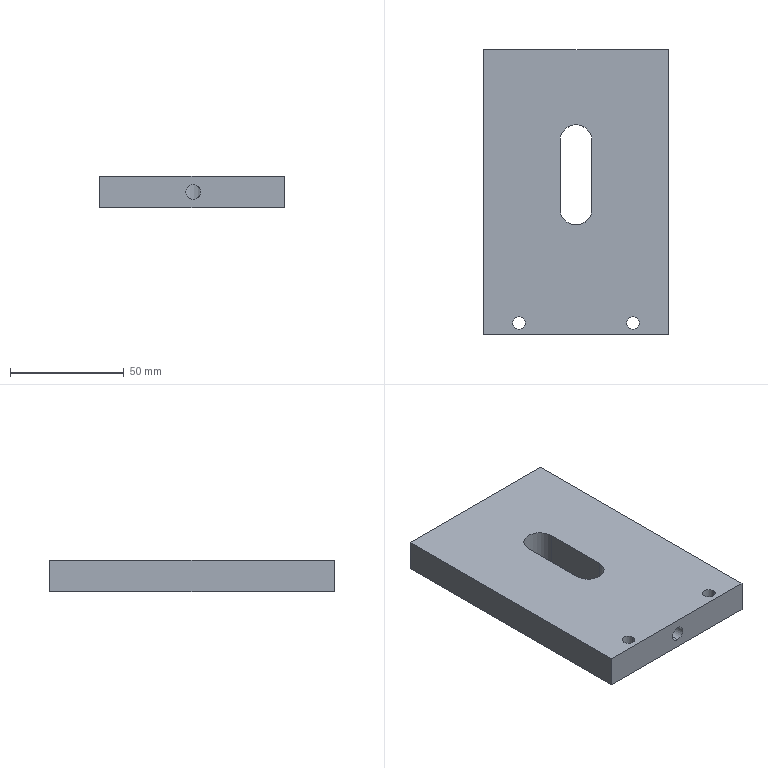Part | SolidWorks | features ICE 2, Cut 1, Extrusion 1, HoleWzd 1 | 1 solid | 24 faces | box 81 x 125 x 14 mm | volume 129784 mm3 | cylinder 12 | plane 8 | cone 4 | commonest cylinder face diameters 5.5 x4 6.8 x4 6.5 x2 14 x2
STEP:
#1=CARTESIAN_POINT('',(62.75,-120.,0.));
#2=VERTEX_POINT('',#1);
#3=CARTESIAN_POINT('',(68.25,-120.,0.));
#4=VERTEX_POINT('',#3);
#5=CARTESIAN_POINT('',(65.5,-120.,0.));
#6=DIRECTION('',(0.,0.,1.));
#7=DIRECTION('',(1.,0.,0.));
#8=AXIS2_PLACEMENT_3D('',#5,#6,#7);
#9=CIRCLE('',#8,2.75);
#10=EDGE_CURVE('',#2,#4,#9,.T.);
#11=ORIENTED_EDGE('',*,*,#10,.F.);
#12=CARTESIAN_POINT('',(62.75,-120.,14.));
#13=VERTEX_POINT('',#12);
#14=CARTESIAN_POINT('',(62.75,-120.,0.));
#15=DIRECTION('',(0.,0.,1.));
#16=VECTOR('',#15,1000.);
#17=LINE('',#14,#16);
#18=EDGE_CURVE('',#2,#13,#17,.T.);
#19=ORIENTED_EDGE('',*,*,#18,.T.);
#20=CARTESIAN_POINT('',(68.25,-120.,14.));
#21=VERTEX_POINT('',#20);
#22=CARTESIAN_POINT('',(65.5,-120.,14.));
#23=DIRECTION('',(0.,0.,1.));
#24=DIRECTION('',(1.,0.,0.));
#25=AXIS2_PLACEMENT_3D('',#22,#23,#24);
#26=CIRCLE('',#25,2.75);
#27=EDGE_CURVE('',#13,#21,#26,.T.);
#28=ORIENTED_EDGE('',*,*,#27,.T.);
#29=CARTESIAN_POINT('',(68.25,-120.,0.));
#30=DIRECTION('',(0.,0.,1.));
#31=VECTOR('',#30,1000.);
#32=LINE('',#29,#31);
#33=EDGE_CURVE('',#4,#21,#32,.T.);
#34=ORIENTED_EDGE('',*,*,#33,.F.);
#35=EDGE_LOOP('',(#11,#19,#28,#34));
#36=FACE_OUTER_BOUND('',#35,.T.);
#37=CARTESIAN_POINT('',(65.5,-120.,0.));
#38=DIRECTION('',(0.,0.,1.));
#39=DIRECTION('',(1.,0.,0.));
#40=AXIS2_PLACEMENT_3D('',#37,#38,#39);
#41=CYLINDRICAL_SURFACE('',#40,2.75);
#42=ADVANCED_FACE('',(#36),#41,.F.);
#43=CARTESIAN_POINT('',(12.75,-120.,0.));
#44=VERTEX_POINT('',#43);
#45=CARTESIAN_POINT('',(18.25,-120.,0.));
#46=VERTEX_POINT('',#45);
#47=CARTESIAN_POINT('',(15.5,-120.,0.));
#48=DIRECTION('',(0.,0.,1.));
#49=DIRECTION('',(1.,0.,0.));
#50=AXIS2_PLACEMENT_3D('',#47,#48,#49);
#51=CIRCLE('',#50,2.75);
#52=EDGE_CURVE('',#44,#46,#51,.T.);
#53=ORIENTED_EDGE('',*,*,#52,.F.);
#54=CARTESIAN_POINT('',(12.75,-120.,14.));
#55=VERTEX_POINT('',#54);
#56=CARTESIAN_POINT('',(12.75,-120.,0.));
#57=DIRECTION('',(0.,0.,1.));
#58=VECTOR('',#57,1000.);
#59=LINE('',#56,#58);
#60=EDGE_CURVE('',#44,#55,#59,.T.);
#61=ORIENTED_EDGE('',*,*,#60,.T.);
#62=CARTESIAN_POINT('',(18.25,-120.,14.));
#63=VERTEX_POINT('',#62);
#64=CARTESIAN_POINT('',(15.5,-120.,14.));
#65=DIRECTION('',(0.,0.,1.));
#66=DIRECTION('',(1.,0.,0.));
#67=AXIS2_PLACEMENT_3D('',#64,#65,#66);
#68=CIRCLE('',#67,2.75);
#69=EDGE_CURVE('',#55,#63,#68,.T.);
#70=ORIENTED_EDGE('',*,*,#69,.T.);
#71=CARTESIAN_POINT('',(18.25,-120.,0.));
#72=DIRECTION('',(0.,0.,1.));
#73=VECTOR('',#72,1000.);
#74=LINE('',#71,#73);
#75=EDGE_CURVE('',#46,#63,#74,.T.);
#76=ORIENTED_EDGE('',*,*,#75,.F.);
#77=EDGE_LOOP('',(#53,#61,#70,#76));
#78=FACE_OUTER_BOUND('',#77,.T.);
#79=CARTESIAN_POINT('',(15.5,-120.,0.));
#80=DIRECTION('',(0.,0.,1.));
#81=DIRECTION('',(1.,0.,0.));
#82=AXIS2_PLACEMENT_3D('',#79,#80,#81);
#83=CYLINDRICAL_SURFACE('',#82,2.75);
#84=ADVANCED_FACE('',(#78),#83,.F.);
#85=CARTESIAN_POINT('',(68.,-22.25,3.6));
#86=VERTEX_POINT('',#85);
#87=CARTESIAN_POINT('',(68.,-22.25,10.4));
#88=VERTEX_POINT('',#87);
#89=CARTESIAN_POINT('',(68.,-22.25,7.));
#90=DIRECTION('',(0.,1.,0.));
#91=DIRECTION('',(0.,0.,1.));
#92=AXIS2_PLACEMENT_3D('',#89,#90,#91);
#93=CIRCLE('',#92,3.4);
#94=EDGE_CURVE('',#86,#88,#93,.T.);
#95=ORIENTED_EDGE('',*,*,#94,.F.);
#96=CARTESIAN_POINT('',(68.,0.,3.6));
#97=VERTEX_POINT('',#96);
#98=CARTESIAN_POINT('',(68.,0.,3.6));
#99=DIRECTION('',(0.,1.,0.));
#100=VECTOR('',#99,1000.);
#101=LINE('',#98,#100);
#102=EDGE_CURVE('',#86,#97,#101,.T.);
#103=ORIENTED_EDGE('',*,*,#102,.T.);
#104=CARTESIAN_POINT('',(68.,0.,10.4));
#105=VERTEX_POINT('',#104);
#106=CARTESIAN_POINT('',(68.,0.,7.));
#107=DIRECTION('',(0.,1.,0.));
#108=DIRECTION('',(0.,0.,1.));
#109=AXIS2_PLACEMENT_3D('',#106,#107,#108);
#110=CIRCLE('',#109,3.4);
#111=EDGE_CURVE('',#97,#105,#110,.T.);
#112=ORIENTED_EDGE('',*,*,#111,.T.);
#113=CARTESIAN_POINT('',(68.,0.,10.4));
#114=DIRECTION('',(0.,1.,0.));
#115=VECTOR('',#114,1000.);
#116=LINE('',#113,#115);
#117=EDGE_CURVE('',#88,#105,#116,.T.);
#118=ORIENTED_EDGE('',*,*,#117,.F.);
#119=EDGE_LOOP('',(#95,#103,#112,#118));
#120=FACE_OUTER_BOUND('',#119,.T.);
#121=CARTESIAN_POINT('',(68.,0.,7.));
#122=DIRECTION('',(0.,1.,0.));
#123=DIRECTION('',(0.,0.,1.));
#124=AXIS2_PLACEMENT_3D('',#121,#122,#123);
#125=CYLINDRICAL_SURFACE('',#124,3.4);
#126=ADVANCED_FACE('',(#120),#125,.F.);
#127=CARTESIAN_POINT('',(68.,-24.293,7.));
#128=VERTEX_POINT('',#127);
#129=CARTESIAN_POINT('',(68.,-22.25,10.4));
#130=DIRECTION('',(0.,0.515,0.8572));
#131=VECTOR('',#130,1000.);
#132=LINE('',#129,#131);
#133=EDGE_CURVE('',#128,#88,#132,.T.);
#134=ORIENTED_EDGE('',*,*,#133,.F.);
#135=CARTESIAN_POINT('',(68.,-22.25,3.6));
#136=DIRECTION('',(0.,0.515,-0.8572));
#137=VECTOR('',#136,1000.);
#138=LINE('',#135,#137);
#139=EDGE_CURVE('',#128,#86,#138,.T.);
#140=ORIENTED_EDGE('',*,*,#139,.T.);
#141=ORIENTED_EDGE('',*,*,#94,.T.);
#142=EDGE_LOOP('',(#134,#140,#141));
#143=FACE_OUTER_BOUND('',#142,.T.);
#144=CARTESIAN_POINT('',(68.,-22.25,7.));
#145=DIRECTION('',(0.,1.,0.));
#146=DIRECTION('',(0.,0.,1.));
#147=AXIS2_PLACEMENT_3D('',#144,#145,#146);
#148=CONICAL_SURFACE('',#147,3.4,1.03);
#149=ADVANCED_FACE('',(#143),#148,.F.);
#150=CARTESIAN_POINT('',(13.,-22.25,3.6));
#151=VERTEX_POINT('',#150);
#152=CARTESIAN_POINT('',(13.,-22.25,10.4));
#153=VERTEX_POINT('',#152);
#154=CARTESIAN_POINT('',(13.,-22.25,7.));
#155=DIRECTION('',(0.,1.,0.));
#156=DIRECTION('',(0.,0.,1.));
#157=AXIS2_PLACEMENT_3D('',#154,#155,#156);
#158=CIRCLE('',#157,3.4);
#159=EDGE_CURVE('',#151,#153,#158,.T.);
#160=ORIENTED_EDGE('',*,*,#159,.F.);
#161=CARTESIAN_POINT('',(13.,0.,3.6));
#162=VERTEX_POINT('',#161);
#163=CARTESIAN_POINT('',(13.,0.,3.6));
#164=DIRECTION('',(0.,1.,0.));
#165=VECTOR('',#164,1000.);
#166=LINE('',#163,#165);
#167=EDGE_CURVE('',#151,#162,#166,.T.);
#168=ORIENTED_EDGE('',*,*,#167,.T.);
#169=CARTESIAN_POINT('',(13.,0.,10.4));
#170=VERTEX_POINT('',#169);
#171=CARTESIAN_POINT('',(13.,0.,7.));
#172=DIRECTION('',(0.,1.,0.));
#173=DIRECTION('',(0.,0.,1.));
#174=AXIS2_PLACEMENT_3D('',#171,#172,#173);
#175=CIRCLE('',#174,3.4);
#176=EDGE_CURVE('',#162,#170,#175,.T.);
#177=ORIENTED_EDGE('',*,*,#176,.T.);
#178=CARTESIAN_POINT('',(13.,0.,10.4));
#179=DIRECTION('',(0.,1.,0.));
#180=VECTOR('',#179,1000.);
#181=LINE('',#178,#180);
#182=EDGE_CURVE('',#153,#170,#181,.T.);
#183=ORIENTED_EDGE('',*,*,#182,.F.);
#184=EDGE_LOOP('',(#160,#168,#177,#183));
#185=FACE_OUTER_BOUND('',#184,.T.);
#186=CARTESIAN_POINT('',(13.,0.,7.));
#187=DIRECTION('',(0.,1.,0.));
#188=DIRECTION('',(0.,0.,1.));
#189=AXIS2_PLACEMENT_3D('',#186,#187,#188);
#190=CYLINDRICAL_SURFACE('',#189,3.4);
#191=ADVANCED_FACE('',(#185),#190,.F.);
#192=CARTESIAN_POINT('',(13.,-24.293,7.));
#193=VERTEX_POINT('',#192);
#194=CARTESIAN_POINT('',(13.,-22.25,10.4));
#195=DIRECTION('',(0.,0.515,0.8572));
#196=VECTOR('',#195,1000.);
#197=LINE('',#194,#196);
#198=EDGE_CURVE('',#193,#153,#197,.T.);
#199=ORIENTED_EDGE('',*,*,#198,.F.);
#200=CARTESIAN_POINT('',(13.,-22.25,3.6));
#201=DIRECTION('',(0.,0.515,-0.8572));
#202=VECTOR('',#201,1000.);
#203=LINE('',#200,#202);
#204=EDGE_CURVE('',#193,#151,#203,.T.);
#205=ORIENTED_EDGE('',*,*,#204,.T.);
#206=ORIENTED_EDGE('',*,*,#159,.T.);
#207=EDGE_LOOP('',(#199,#205,#206));
#208=FACE_OUTER_BOUND('',#207,.T.);
#209=CARTESIAN_POINT('',(13.,-22.25,7.));
#210=DIRECTION('',(0.,1.,0.));
#211=DIRECTION('',(0.,0.,1.));
#212=AXIS2_PLACEMENT_3D('',#209,#210,#211);
#213=CONICAL_SURFACE('',#212,3.4,1.03);
#214=ADVANCED_FACE('',(#208),#213,.F.);
#215=CARTESIAN_POINT('',(41.,-76.982,3.75));
#216=VERTEX_POINT('',#215);
#217=CARTESIAN_POINT('',(41.,-76.982,10.25));
#218=VERTEX_POINT('',#217);
#219=CARTESIAN_POINT('',(41.,-76.982,3.75));
#220=CARTESIAN_POINT('',(40.784,-76.998,3.75));
#221=CARTESIAN_POINT('',(40.571,-77.003,3.771));
#222=CARTESIAN_POINT('',(40.152,-76.994,3.855));
#223=CARTESIAN_POINT('',(39.944,-76.981,3.919));
#224=CARTESIAN_POINT('',(39.55,-76.938,4.083));
#225=CARTESIAN_POINT('',(39.364,-76.909,4.184));
#226=CARTESIAN_POINT('',(39.01,-76.842,4.421));
#227=CARTESIAN_POINT('',(38.846,-76.804,4.557));
#228=CARTESIAN_POINT('',(38.55,-76.725,4.855));
#229=CARTESIAN_POINT('',(38.415,-76.683,5.019));
#230=CARTESIAN_POINT('',(38.18,-76.605,5.371));
#231=CARTESIAN_POINT('',(38.081,-76.569,5.556));
#232=CARTESIAN_POINT('',(37.918,-76.507,5.947));
#233=CARTESIAN_POINT('',(37.855,-76.481,6.154));
#234=CARTESIAN_POINT('',(37.771,-76.446,6.572));
#235=CARTESIAN_POINT('',(37.75,-76.437,6.784));
#236=CARTESIAN_POINT('',(37.75,-76.437,7.213));
#237=CARTESIAN_POINT('',(37.772,-76.447,7.43));
#238=CARTESIAN_POINT('',(37.855,-76.481,7.848));
#239=CARTESIAN_POINT('',(37.918,-76.507,8.053));
#240=CARTESIAN_POINT('',(38.082,-76.57,8.447));
#241=CARTESIAN_POINT('',(38.182,-76.606,8.633));
#242=CARTESIAN_POINT('',(38.416,-76.684,8.983));
#243=CARTESIAN_POINT('',(38.552,-76.725,9.148));
#244=CARTESIAN_POINT('',(38.849,-76.804,9.446));
#245=CARTESIAN_POINT('',(39.012,-76.842,9.58));
#246=CARTESIAN_POINT('',(39.365,-76.91,9.817));
#247=CARTESIAN_POINT('',(39.554,-76.939,9.918));
#248=CARTESIAN_POINT('',(39.945,-76.981,10.081));
#249=CARTESIAN_POINT('',(40.15,-76.994,10.144));
#250=CARTESIAN_POINT('',(40.574,-77.003,10.229));
#251=CARTESIAN_POINT('',(40.787,-76.997,10.25));
#252=CARTESIAN_POINT('',(41.,-76.982,10.25));
#253=B_SPLINE_CURVE_WITH_KNOTS('',3,(#219,#220,#221,#222,#223,#224,#225,#226,#227,#228,#229,#230,#231,#232,#233,#234,#235,#236,#237,#238,#239,#240,#241,#242,#243,#244,#245,#246,#247,#248,#249,#250,#251,#252),.UNSPECIFIED.,.F.,.F.,(4,2,2,2,2,2,2,2,2,2,2,2,2,2,2,2,4),(0.,0.0006404,0.001281,0.001921,0.002561,0.003202,0.003842,0.004483,0.005123,0.005763,0.006404,0.007044,0.007684,0.008325,0.008965,0.009606,0.01025),.UNSPECIFIED.);
#254=EDGE_CURVE('',#216,#218,#253,.T.);
#255=ORIENTED_EDGE('',*,*,#254,.T.);
#256=CARTESIAN_POINT('',(41.,-125.,10.25));
#257=VERTEX_POINT('',#256);
#258=CARTESIAN_POINT('',(41.,0.001,10.25));
#259=DIRECTION('',(0.,-1.,0.));
#260=VECTOR('',#259,1000.);
#261=LINE('',#258,#260);
#262=EDGE_CURVE('',#218,#257,#261,.T.);
#263=ORIENTED_EDGE('',*,*,#262,.T.);
#264=CARTESIAN_POINT('',(41.,-125.,3.75));
#265=VERTEX_POINT('',#264);
#266=CARTESIAN_POINT('',(41.,-125.,7.));
#267=DIRECTION('',(0.,-1.,0.));
#268=DIRECTION('',(0.,0.,-1.));
#269=AXIS2_PLACEMENT_3D('',#266,#267,#268);
#270=CIRCLE('',#269,3.25);
#271=EDGE_CURVE('',#257,#265,#270,.T.);
#272=ORIENTED_EDGE('',*,*,#271,.T.);
#273=CARTESIAN_POINT('',(41.,0.001,3.75));
#274=DIRECTION('',(0.,-1.,0.));
#275=VECTOR('',#274,1000.);
#276=LINE('',#273,#275);
#277=EDGE_CURVE('',#216,#265,#276,.T.);
#278=ORIENTED_EDGE('',*,*,#277,.F.);
#279=EDGE_LOOP('',(#255,#263,#272,#278));
#280=FACE_OUTER_BOUND('',#279,.T.);
#281=CARTESIAN_POINT('',(41.,0.001,7.));
#282=DIRECTION('',(0.,-1.,0.));
#283=DIRECTION('',(0.,0.,-1.));
#284=AXIS2_PLACEMENT_3D('',#281,#282,#283);
#285=CYLINDRICAL_SURFACE('',#284,3.25);
#286=ADVANCED_FACE('',(#280),#285,.F.);
#287=CARTESIAN_POINT('',(0.,0.,0.));
#288=VERTEX_POINT('',#287);
#289=CARTESIAN_POINT('',(0.,-125.,0.));
#290=VERTEX_POINT('',#289);
#291=CARTESIAN_POINT('',(0.,0.,0.));
#292=DIRECTION('',(0.,-1.,0.));
#293=VECTOR('',#292,1000.);
#294=LINE('',#291,#293);
#295=EDGE_CURVE('',#288,#290,#294,.T.);
#296=ORIENTED_EDGE('',*,*,#295,.T.);
#297=CARTESIAN_POINT('',(0.,-125.,14.));
#298=VERTEX_POINT('',#297);
#299=CARTESIAN_POINT('',(0.,-125.,14.));
#300=DIRECTION('',(0.,0.,-1.));
#301=VECTOR('',#300,1000.);
#302=LINE('',#299,#301);
#303=EDGE_CURVE('',#298,#290,#302,.T.);
#304=ORIENTED_EDGE('',*,*,#303,.F.);
#305=CARTESIAN_POINT('',(0.,0.,14.));
#306=VERTEX_POINT('',#305);
#307=CARTESIAN_POINT('',(0.,0.,14.));
#308=DIRECTION('',(0.,-1.,0.));
#309=VECTOR('',#308,1000.);
#310=LINE('',#307,#309);
#311=EDGE_CURVE('',#306,#298,#310,.T.);
#312=ORIENTED_EDGE('',*,*,#311,.F.);
#313=CARTESIAN_POINT('',(0.,0.,14.));
#314=DIRECTION('',(0.,0.,-1.));
#315=VECTOR('',#314,1000.);
#316=LINE('',#313,#315);
#317=EDGE_CURVE('',#306,#288,#316,.T.);
#318=ORIENTED_EDGE('',*,*,#317,.T.);
#319=EDGE_LOOP('',(#296,#304,#312,#318));
#320=FACE_OUTER_BOUND('',#319,.T.);
#321=CARTESIAN_POINT('',(0.,0.,14.));
#322=DIRECTION('',(1.,0.,0.));
#323=DIRECTION('',(0.,1.,0.));
#324=AXIS2_PLACEMENT_3D('',#321,#322,#323);
#325=PLANE('',#324);
#326=ADVANCED_FACE('',(#320),#325,.F.);
#327=CARTESIAN_POINT('',(41.,-125.,7.));
#328=DIRECTION('',(0.,-1.,0.));
#329=DIRECTION('',(0.,0.,-1.));
#330=AXIS2_PLACEMENT_3D('',#327,#328,#329);
#331=CIRCLE('',#330,3.25);
#332=EDGE_CURVE('',#265,#257,#331,.T.);
#333=ORIENTED_EDGE('',*,*,#332,.F.);
#334=ORIENTED_EDGE('',*,*,#271,.F.);
#335=EDGE_LOOP('',(#333,#334));
#336=FACE_BOUND('',#335,.T.);
#337=CARTESIAN_POINT('',(81.,-125.,0.));
#338=VERTEX_POINT('',#337);
#339=CARTESIAN_POINT('',(0.,-125.,0.));
#340=DIRECTION('',(1.,0.,0.));
#341=VECTOR('',#340,1000.);
#342=LINE('',#339,#341);
#343=EDGE_CURVE('',#290,#338,#342,.T.);
#344=ORIENTED_EDGE('',*,*,#343,.T.);
#345=CARTESIAN_POINT('',(81.,-125.,14.));
#346=VERTEX_POINT('',#345);
#347=CARTESIAN_POINT('',(81.,-125.,14.));
#348=DIRECTION('',(0.,0.,-1.));
#349=VECTOR('',#348,1000.);
#350=LINE('',#347,#349);
#351=EDGE_CURVE('',#346,#338,#350,.T.);
#352=ORIENTED_EDGE('',*,*,#351,.F.);
#353=CARTESIAN_POINT('',(0.,-125.,14.));
#354=DIRECTION('',(1.,0.,0.));
#355=VECTOR('',#354,1000.);
#356=LINE('',#353,#355);
#357=EDGE_CURVE('',#298,#346,#356,.T.);
#358=ORIENTED_EDGE('',*,*,#357,.F.);
#359=ORIENTED_EDGE('',*,*,#303,.T.);
#360=EDGE_LOOP('',(#344,#352,#358,#359));
#361=FACE_OUTER_BOUND('',#360,.T.);
#362=CARTESIAN_POINT('',(0.,-125.,14.));
#363=DIRECTION('',(0.,1.,0.));
#364=DIRECTION('',(0.,0.,1.));
#365=AXIS2_PLACEMENT_3D('',#362,#363,#364);
#366=PLANE('',#365);
#367=ADVANCED_FACE('',(#336,#361),#366,.F.);
#368=CARTESIAN_POINT('',(81.,0.,0.));
#369=VERTEX_POINT('',#368);
#370=CARTESIAN_POINT('',(81.,0.,0.));
#371=DIRECTION('',(0.,1.,0.));
#372=VECTOR('',#371,1000.);
#373=LINE('',#370,#372);
#374=EDGE_CURVE('',#338,#369,#373,.T.);
#375=ORIENTED_EDGE('',*,*,#374,.T.);
#376=CARTESIAN_POINT('',(81.,0.,14.));
#377=VERTEX_POINT('',#376);
#378=CARTESIAN_POINT('',(81.,0.,14.));
#379=DIRECTION('',(0.,0.,-1.));
#380=VECTOR('',#379,1000.);
#381=LINE('',#378,#380);
#382=EDGE_CURVE('',#377,#369,#381,.T.);
#383=ORIENTED_EDGE('',*,*,#382,.F.);
#384=CARTESIAN_POINT('',(81.,0.,14.));
#385=DIRECTION('',(0.,1.,0.));
#386=VECTOR('',#385,1000.);
#387=LINE('',#384,#386);
#388=EDGE_CURVE('',#346,#377,#387,.T.);
#389=ORIENTED_EDGE('',*,*,#388,.F.);
#390=ORIENTED_EDGE('',*,*,#351,.T.);
#391=EDGE_LOOP('',(#375,#383,#389,#390));
#392=FACE_OUTER_BOUND('',#391,.T.);
#393=CARTESIAN_POINT('',(81.,0.,14.));
#394=DIRECTION('',(-1.,0.,0.));
#395=DIRECTION('',(0.,-1.,0.));
#396=AXIS2_PLACEMENT_3D('',#393,#394,#395);
#397=PLANE('',#396);
#398=ADVANCED_FACE('',(#392),#397,.F.);
#399=CARTESIAN_POINT('',(68.,0.,7.));
#400=DIRECTION('',(0.,1.,0.));
#401=DIRECTION('',(0.,0.,1.));
#402=AXIS2_PLACEMENT_3D('',#399,#400,#401);
#403=CIRCLE('',#402,3.4);
#404=EDGE_CURVE('',#105,#97,#403,.T.);
#405=ORIENTED_EDGE('',*,*,#404,.F.);
#406=ORIENTED_EDGE('',*,*,#111,.F.);
#407=EDGE_LOOP('',(#405,#406));
#408=FACE_BOUND('',#407,.T.);
#409=CARTESIAN_POINT('',(13.,0.,7.));
#410=DIRECTION('',(0.,1.,0.));
#411=DIRECTION('',(0.,0.,1.));
#412=AXIS2_PLACEMENT_3D('',#409,#410,#411);
#413=CIRCLE('',#412,3.4);
#414=EDGE_CURVE('',#170,#162,#413,.T.);
#415=ORIENTED_EDGE('',*,*,#414,.F.);
#416=ORIENTED_EDGE('',*,*,#176,.F.);
#417=EDGE_LOOP('',(#415,#416));
#418=FACE_BOUND('',#417,.T.);
#419=CARTESIAN_POINT('',(0.,0.,0.));
#420=DIRECTION('',(-1.,0.,0.));
#421=VECTOR('',#420,1000.);
#422=LINE('',#419,#421);
#423=EDGE_CURVE('',#369,#288,#422,.T.);
#424=ORIENTED_EDGE('',*,*,#423,.T.);
#425=ORIENTED_EDGE('',*,*,#317,.F.);
#426=CARTESIAN_POINT('',(0.,0.,14.));
#427=DIRECTION('',(-1.,0.,0.));
#428=VECTOR('',#427,1000.);
#429=LINE('',#426,#428);
#430=EDGE_CURVE('',#377,#306,#429,.T.);
#431=ORIENTED_EDGE('',*,*,#430,.F.);
#432=ORIENTED_EDGE('',*,*,#382,.T.);
#433=EDGE_LOOP('',(#424,#425,#431,#432));
#434=FACE_OUTER_BOUND('',#433,.T.);
#435=CARTESIAN_POINT('',(0.,0.,14.));
#436=DIRECTION('',(0.,-1.,0.));
#437=DIRECTION('',(0.,0.,-1.));
#438=AXIS2_PLACEMENT_3D('',#435,#436,#437);
#439=PLANE('',#438);
#440=ADVANCED_FACE('',(#408,#418,#434),#439,.F.);
#441=CARTESIAN_POINT('',(65.5,-120.,14.));
#442=DIRECTION('',(0.,0.,1.));
#443=DIRECTION('',(1.,0.,0.));
#444=AXIS2_PLACEMENT_3D('',#441,#442,#443);
#445=CIRCLE('',#444,2.75);
#446=EDGE_CURVE('',#21,#13,#445,.T.);
#447=ORIENTED_EDGE('',*,*,#446,.F.);
#448=ORIENTED_EDGE('',*,*,#27,.F.);
#449=EDGE_LOOP('',(#447,#448));
#450=FACE_BOUND('',#449,.T.);
#451=CARTESIAN_POINT('',(15.5,-120.,14.));
#452=DIRECTION('',(0.,0.,1.));
#453=DIRECTION('',(1.,0.,0.));
#454=AXIS2_PLACEMENT_3D('',#451,#452,#453);
#455=CIRCLE('',#454,2.75);
#456=EDGE_CURVE('',#63,#55,#455,.T.);
#457=ORIENTED_EDGE('',*,*,#456,.F.);
#458=ORIENTED_EDGE('',*,*,#69,.F.);
#459=EDGE_LOOP('',(#457,#458));
#460=FACE_BOUND('',#459,.T.);
#461=CARTESIAN_POINT('',(33.5,-70.,14.));
#462=VERTEX_POINT('',#461);
#463=CARTESIAN_POINT('',(47.5,-70.,14.));
#464=VERTEX_POINT('',#463);
#465=CARTESIAN_POINT('',(40.5,-70.,14.));
#466=DIRECTION('',(0.,0.,1.));
#467=DIRECTION('',(1.,0.,0.));
#468=AXIS2_PLACEMENT_3D('',#465,#466,#467);
#469=CIRCLE('',#468,7.);
#470=EDGE_CURVE('',#462,#464,#469,.T.);
#471=ORIENTED_EDGE('',*,*,#470,.F.);
#472=CARTESIAN_POINT('',(33.5,-40.,14.));
#473=VERTEX_POINT('',#472);
#474=CARTESIAN_POINT('',(33.5,-70.,14.));
#475=DIRECTION('',(0.,-1.,0.));
#476=VECTOR('',#475,1000.);
#477=LINE('',#474,#476);
#478=EDGE_CURVE('',#473,#462,#477,.T.);
#479=ORIENTED_EDGE('',*,*,#478,.F.);
#480=CARTESIAN_POINT('',(47.5,-40.,14.));
#481=VERTEX_POINT('',#480);
#482=CARTESIAN_POINT('',(40.5,-40.,14.));
#483=DIRECTION('',(0.,0.,1.));
#484=DIRECTION('',(1.,0.,0.));
#485=AXIS2_PLACEMENT_3D('',#482,#483,#484);
#486=CIRCLE('',#485,7.);
#487=EDGE_CURVE('',#481,#473,#486,.T.);
#488=ORIENTED_EDGE('',*,*,#487,.F.);
#489=CARTESIAN_POINT('',(47.5,-70.,14.));
#490=DIRECTION('',(0.,1.,0.));
#491=VECTOR('',#490,1000.);
#492=LINE('',#489,#491);
#493=EDGE_CURVE('',#464,#481,#492,.T.);
#494=ORIENTED_EDGE('',*,*,#493,.F.);
#495=EDGE_LOOP('',(#471,#479,#488,#494));
#496=FACE_BOUND('',#495,.T.);
#497=ORIENTED_EDGE('',*,*,#311,.T.);
#498=ORIENTED_EDGE('',*,*,#357,.T.);
#499=ORIENTED_EDGE('',*,*,#388,.T.);
#500=ORIENTED_EDGE('',*,*,#430,.T.);
#501=EDGE_LOOP('',(#497,#498,#499,#500));
#502=FACE_OUTER_BOUND('',#501,.T.);
#503=CARTESIAN_POINT('',(0.,0.,14.));
#504=DIRECTION('',(0.,0.,1.));
#505=DIRECTION('',(1.,0.,0.));
#506=AXIS2_PLACEMENT_3D('',#503,#504,#505);
#507=PLANE('',#506);
#508=ADVANCED_FACE('',(#450,#460,#496,#502),#507,.T.);
#509=CARTESIAN_POINT('',(65.5,-120.,0.));
#510=DIRECTION('',(0.,0.,1.));
#511=DIRECTION('',(1.,0.,0.));
#512=AXIS2_PLACEMENT_3D('',#509,#510,#511);
#513=CIRCLE('',#512,2.75);
#514=EDGE_CURVE('',#4,#2,#513,.T.);
#515=ORIENTED_EDGE('',*,*,#514,.T.);
#516=ORIENTED_EDGE('',*,*,#10,.T.);
#517=EDGE_LOOP('',(#515,#516));
#518=FACE_BOUND('',#517,.T.);
#519=CARTESIAN_POINT('',(15.5,-120.,0.));
#520=DIRECTION('',(0.,0.,1.));
#521=DIRECTION('',(1.,0.,0.));
#522=AXIS2_PLACEMENT_3D('',#519,#520,#521);
#523=CIRCLE('',#522,2.75);
#524=EDGE_CURVE('',#46,#44,#523,.T.);
#525=ORIENTED_EDGE('',*,*,#524,.T.);
#526=ORIENTED_EDGE('',*,*,#52,.T.);
#527=EDGE_LOOP('',(#525,#526));
#528=FACE_BOUND('',#527,.T.);
#529=CARTESIAN_POINT('',(33.5,-40.,0.));
#530=VERTEX_POINT('',#529);
#531=CARTESIAN_POINT('',(33.5,-70.,0.));
#532=VERTEX_POINT('',#531);
#533=CARTESIAN_POINT('',(33.5,-70.,0.));
#534=DIRECTION('',(0.,-1.,0.));
#535=VECTOR('',#534,1000.);
#536=LINE('',#533,#535);
#537=EDGE_CURVE('',#530,#532,#536,.T.);
#538=ORIENTED_EDGE('',*,*,#537,.T.);
#539=CARTESIAN_POINT('',(47.5,-70.,0.));
#540=VERTEX_POINT('',#539);
#541=CARTESIAN_POINT('',(40.5,-70.,0.));
#542=DIRECTION('',(0.,0.,1.));
#543=DIRECTION('',(1.,0.,0.));
#544=AXIS2_PLACEMENT_3D('',#541,#542,#543);
#545=CIRCLE('',#544,7.);
#546=EDGE_CURVE('',#532,#540,#545,.T.);
#547=ORIENTED_EDGE('',*,*,#546,.T.);
#548=CARTESIAN_POINT('',(47.5,-40.,0.));
#549=VERTEX_POINT('',#548);
#550=CARTESIAN_POINT('',(47.5,-70.,0.));
#551=DIRECTION('',(0.,1.,0.));
#552=VECTOR('',#551,1000.);
#553=LINE('',#550,#552);
#554=EDGE_CURVE('',#540,#549,#553,.T.);
#555=ORIENTED_EDGE('',*,*,#554,.T.);
#556=CARTESIAN_POINT('',(40.5,-40.,0.));
#557=DIRECTION('',(0.,0.,1.));
#558=DIRECTION('',(1.,0.,0.));
#559=AXIS2_PLACEMENT_3D('',#556,#557,#558);
#560=CIRCLE('',#559,7.);
#561=EDGE_CURVE('',#549,#530,#560,.T.);
#562=ORIENTED_EDGE('',*,*,#561,.T.);
#563=EDGE_LOOP('',(#538,#547,#555,#562));
#564=FACE_BOUND('',#563,.T.);
#565=ORIENTED_EDGE('',*,*,#295,.F.);
#566=ORIENTED_EDGE('',*,*,#423,.F.);
#567=ORIENTED_EDGE('',*,*,#374,.F.);
#568=ORIENTED_EDGE('',*,*,#343,.F.);
#569=EDGE_LOOP('',(#565,#566,#567,#568));
#570=FACE_OUTER_BOUND('',#569,.T.);
#571=CARTESIAN_POINT('',(0.,0.,0.));
#572=DIRECTION('',(0.,0.,1.));
#573=DIRECTION('',(1.,0.,0.));
#574=AXIS2_PLACEMENT_3D('',#571,#572,#573);
#575=PLANE('',#574);
#576=ADVANCED_FACE('',(#518,#528,#564,#570),#575,.F.);
#577=ORIENTED_EDGE('',*,*,#254,.F.);
#578=CARTESIAN_POINT('',(41.,-76.982,10.25));
#579=CARTESIAN_POINT('',(41.216,-76.967,10.25));
#580=CARTESIAN_POINT('',(41.436,-76.94,10.228));
#581=CARTESIAN_POINT('',(41.857,-76.871,10.142));
#582=CARTESIAN_POINT('',(42.06,-76.827,10.08));
#583=CARTESIAN_POINT('',(42.454,-76.725,9.914));
#584=CARTESIAN_POINT('',(42.64,-76.668,9.814));
#585=CARTESIAN_POINT('',(42.986,-76.546,9.581));
#586=CARTESIAN_POINT('',(43.149,-76.481,9.447));
#587=CARTESIAN_POINT('',(43.444,-76.353,9.152));
#588=CARTESIAN_POINT('',(43.576,-76.289,8.992));
#589=CARTESIAN_POINT('',(43.81,-76.169,8.646));
#590=CARTESIAN_POINT('',(43.913,-76.113,8.458));
#591=CARTESIAN_POINT('',(44.077,-76.018,8.068));
#592=CARTESIAN_POINT('',(44.14,-75.979,7.865));
#593=CARTESIAN_POINT('',(44.227,-75.925,7.441));
#594=CARTESIAN_POINT('',(44.25,-75.911,7.221));
#595=CARTESIAN_POINT('',(44.25,-75.911,6.788));
#596=CARTESIAN_POINT('',(44.229,-75.924,6.57));
#597=CARTESIAN_POINT('',(44.142,-75.978,6.143));
#598=CARTESIAN_POINT('',(44.079,-76.017,5.938));
#599=CARTESIAN_POINT('',(43.914,-76.112,5.545));
#600=CARTESIAN_POINT('',(43.812,-76.168,5.357));
#601=CARTESIAN_POINT('',(43.578,-76.288,5.01));
#602=CARTESIAN_POINT('',(43.444,-76.353,4.848));
#603=CARTESIAN_POINT('',(43.148,-76.482,4.552));
#604=CARTESIAN_POINT('',(42.987,-76.546,4.42));
#605=CARTESIAN_POINT('',(42.641,-76.667,4.187));
#606=CARTESIAN_POINT('',(42.453,-76.725,4.085));
#607=CARTESIAN_POINT('',(42.062,-76.826,3.921));
#608=CARTESIAN_POINT('',(41.86,-76.87,3.858));
#609=CARTESIAN_POINT('',(41.439,-76.94,3.773));
#610=CARTESIAN_POINT('',(41.219,-76.966,3.75));
#611=CARTESIAN_POINT('',(41.,-76.982,3.75));
#612=B_SPLINE_CURVE_WITH_KNOTS('',3,(#578,#579,#580,#581,#582,#583,#584,#585,#586,#587,#588,#589,#590,#591,#592,#593,#594,#595,#596,#597,#598,#599,#600,#601,#602,#603,#604,#605,#606,#607,#608,#609,#610,#611),.UNSPECIFIED.,.F.,.F.,(4,2,2,2,2,2,2,2,2,2,2,2,2,2,2,2,4),(0.01025,0.0109,0.01155,0.0122,0.01285,0.0135,0.01415,0.0148,0.01545,0.0161,0.01675,0.0174,0.01805,0.0187,0.01935,0.02,0.02065),.UNSPECIFIED.);
#613=EDGE_CURVE('',#218,#216,#612,.T.);
#614=ORIENTED_EDGE('',*,*,#613,.F.);
#615=EDGE_LOOP('',(#577,#614));
#616=FACE_BOUND('',#615,.T.);
#617=ORIENTED_EDGE('',*,*,#470,.T.);
#618=CARTESIAN_POINT('',(47.5,-70.,0.));
#619=DIRECTION('',(0.,0.,1.));
#620=VECTOR('',#619,1000.);
#621=LINE('',#618,#620);
#622=EDGE_CURVE('',#540,#464,#621,.T.);
#623=ORIENTED_EDGE('',*,*,#622,.F.);
#624=ORIENTED_EDGE('',*,*,#546,.F.);
#625=CARTESIAN_POINT('',(33.5,-70.,0.));
#626=DIRECTION('',(0.,0.,1.));
#627=VECTOR('',#626,1000.);
#628=LINE('',#625,#627);
#629=EDGE_CURVE('',#532,#462,#628,.T.);
#630=ORIENTED_EDGE('',*,*,#629,.T.);
#631=EDGE_LOOP('',(#617,#623,#624,#630));
#632=FACE_OUTER_BOUND('',#631,.T.);
#633=CARTESIAN_POINT('',(40.5,-70.,0.));
#634=DIRECTION('',(0.,0.,1.));
#635=DIRECTION('',(1.,0.,0.));
#636=AXIS2_PLACEMENT_3D('',#633,#634,#635);
#637=CYLINDRICAL_SURFACE('',#636,7.);
#638=ADVANCED_FACE('',(#616,#632),#637,.F.);
#639=ORIENTED_EDGE('',*,*,#478,.T.);
#640=ORIENTED_EDGE('',*,*,#629,.F.);
#641=ORIENTED_EDGE('',*,*,#537,.F.);
#642=CARTESIAN_POINT('',(33.5,-40.,0.));
#643=DIRECTION('',(0.,0.,1.));
#644=VECTOR('',#643,1000.);
#645=LINE('',#642,#644);
#646=EDGE_CURVE('',#530,#473,#645,.T.);
#647=ORIENTED_EDGE('',*,*,#646,.T.);
#648=EDGE_LOOP('',(#639,#640,#641,#647));
#649=FACE_OUTER_BOUND('',#648,.T.);
#650=CARTESIAN_POINT('',(33.5,-70.,0.));
#651=DIRECTION('',(-1.,0.,0.));
#652=DIRECTION('',(0.,-1.,0.));
#653=AXIS2_PLACEMENT_3D('',#650,#651,#652);
#654=PLANE('',#653);
#655=ADVANCED_FACE('',(#649),#654,.F.);
#656=ORIENTED_EDGE('',*,*,#487,.T.);
#657=ORIENTED_EDGE('',*,*,#646,.F.);
#658=ORIENTED_EDGE('',*,*,#561,.F.);
#659=CARTESIAN_POINT('',(47.5,-40.,0.));
#660=DIRECTION('',(0.,0.,1.));
#661=VECTOR('',#660,1000.);
#662=LINE('',#659,#661);
#663=EDGE_CURVE('',#549,#481,#662,.T.);
#664=ORIENTED_EDGE('',*,*,#663,.T.);
#665=EDGE_LOOP('',(#656,#657,#658,#664));
#666=FACE_OUTER_BOUND('',#665,.T.);
#667=CARTESIAN_POINT('',(40.5,-40.,0.));
#668=DIRECTION('',(0.,0.,1.));
#669=DIRECTION('',(1.,0.,0.));
#670=AXIS2_PLACEMENT_3D('',#667,#668,#669);
#671=CYLINDRICAL_SURFACE('',#670,7.);
#672=ADVANCED_FACE('',(#666),#671,.F.);
#673=ORIENTED_EDGE('',*,*,#493,.T.);
#674=ORIENTED_EDGE('',*,*,#663,.F.);
#675=ORIENTED_EDGE('',*,*,#554,.F.);
#676=ORIENTED_EDGE('',*,*,#622,.T.);
#677=EDGE_LOOP('',(#673,#674,#675,#676));
#678=FACE_OUTER_BOUND('',#677,.T.);
#679=CARTESIAN_POINT('',(47.5,-70.,0.));
#680=DIRECTION('',(1.,0.,0.));
#681=DIRECTION('',(0.,1.,0.));
#682=AXIS2_PLACEMENT_3D('',#679,#680,#681);
#683=PLANE('',#682);
#684=ADVANCED_FACE('',(#678),#683,.F.);
#685=ORIENTED_EDGE('',*,*,#262,.F.);
#686=ORIENTED_EDGE('',*,*,#613,.T.);
#687=ORIENTED_EDGE('',*,*,#277,.T.);
#688=ORIENTED_EDGE('',*,*,#332,.T.);
#689=EDGE_LOOP('',(#685,#686,#687,#688));
#690=FACE_OUTER_BOUND('',#689,.T.);
#691=CARTESIAN_POINT('',(41.,0.001,7.));
#692=DIRECTION('',(0.,-1.,0.));
#693=DIRECTION('',(0.,0.,-1.));
#694=AXIS2_PLACEMENT_3D('',#691,#692,#693);
#695=CYLINDRICAL_SURFACE('',#694,3.25);
#696=ADVANCED_FACE('',(#690),#695,.F.);
#697=ORIENTED_EDGE('',*,*,#204,.F.);
#698=ORIENTED_EDGE('',*,*,#198,.T.);
#699=CARTESIAN_POINT('',(13.,-22.25,7.));
#700=DIRECTION('',(0.,1.,0.));
#701=DIRECTION('',(0.,0.,1.));
#702=AXIS2_PLACEMENT_3D('',#699,#700,#701);
#703=CIRCLE('',#702,3.4);
#704=EDGE_CURVE('',#153,#151,#703,.T.);
#705=ORIENTED_EDGE('',*,*,#704,.T.);
#706=EDGE_LOOP('',(#697,#698,#705));
#707=FACE_OUTER_BOUND('',#706,.T.);
#708=CARTESIAN_POINT('',(13.,-22.25,7.));
#709=DIRECTION('',(0.,1.,0.));
#710=DIRECTION('',(0.,0.,1.));
#711=AXIS2_PLACEMENT_3D('',#708,#709,#710);
#712=CONICAL_SURFACE('',#711,3.4,1.03);
#713=ADVANCED_FACE('',(#707),#712,.F.);
#714=ORIENTED_EDGE('',*,*,#167,.F.);
#715=ORIENTED_EDGE('',*,*,#704,.F.);
#716=ORIENTED_EDGE('',*,*,#182,.T.);
#717=ORIENTED_EDGE('',*,*,#414,.T.);
#718=EDGE_LOOP('',(#714,#715,#716,#717));
#719=FACE_OUTER_BOUND('',#718,.T.);
#720=CARTESIAN_POINT('',(13.,0.,7.));
#721=DIRECTION('',(0.,1.,0.));
#722=DIRECTION('',(0.,0.,1.));
#723=AXIS2_PLACEMENT_3D('',#720,#721,#722);
#724=CYLINDRICAL_SURFACE('',#723,3.4);
#725=ADVANCED_FACE('',(#719),#724,.F.);
#726=ORIENTED_EDGE('',*,*,#139,.F.);
#727=ORIENTED_EDGE('',*,*,#133,.T.);
#728=CARTESIAN_POINT('',(68.,-22.25,7.));
#729=DIRECTION('',(0.,1.,0.));
#730=DIRECTION('',(0.,0.,1.));
#731=AXIS2_PLACEMENT_3D('',#728,#729,#730);
#732=CIRCLE('',#731,3.4);
#733=EDGE_CURVE('',#88,#86,#732,.T.);
#734=ORIENTED_EDGE('',*,*,#733,.T.);
#735=EDGE_LOOP('',(#726,#727,#734));
#736=FACE_OUTER_BOUND('',#735,.T.);
#737=CARTESIAN_POINT('',(68.,-22.25,7.));
#738=DIRECTION('',(0.,1.,0.));
#739=DIRECTION('',(0.,0.,1.));
#740=AXIS2_PLACEMENT_3D('',#737,#738,#739);
#741=CONICAL_SURFACE('',#740,3.4,1.03);
#742=ADVANCED_FACE('',(#736),#741,.F.);
#743=ORIENTED_EDGE('',*,*,#102,.F.);
#744=ORIENTED_EDGE('',*,*,#733,.F.);
#745=ORIENTED_EDGE('',*,*,#117,.T.);
#746=ORIENTED_EDGE('',*,*,#404,.T.);
#747=EDGE_LOOP('',(#743,#744,#745,#746));
#748=FACE_OUTER_BOUND('',#747,.T.);
#749=CARTESIAN_POINT('',(68.,0.,7.));
#750=DIRECTION('',(0.,1.,0.));
#751=DIRECTION('',(0.,0.,1.));
#752=AXIS2_PLACEMENT_3D('',#749,#750,#751);
#753=CYLINDRICAL_SURFACE('',#752,3.4);
#754=ADVANCED_FACE('',(#748),#753,.F.);
#755=ORIENTED_EDGE('',*,*,#60,.F.);
#756=ORIENTED_EDGE('',*,*,#524,.F.);
#757=ORIENTED_EDGE('',*,*,#75,.T.);
#758=ORIENTED_EDGE('',*,*,#456,.T.);
#759=EDGE_LOOP('',(#755,#756,#757,#758));
#760=FACE_OUTER_BOUND('',#759,.T.);
#761=CARTESIAN_POINT('',(15.5,-120.,0.));
#762=DIRECTION('',(0.,0.,1.));
#763=DIRECTION('',(1.,0.,0.));
#764=AXIS2_PLACEMENT_3D('',#761,#762,#763);
#765=CYLINDRICAL_SURFACE('',#764,2.75);
#766=ADVANCED_FACE('',(#760),#765,.F.);
#767=ORIENTED_EDGE('',*,*,#18,.F.);
#768=ORIENTED_EDGE('',*,*,#514,.F.);
#769=ORIENTED_EDGE('',*,*,#33,.T.);
#770=ORIENTED_EDGE('',*,*,#446,.T.);
#771=EDGE_LOOP('',(#767,#768,#769,#770));
#772=FACE_OUTER_BOUND('',#771,.T.);
#773=CARTESIAN_POINT('',(65.5,-120.,0.));
#774=DIRECTION('',(0.,0.,1.));
#775=DIRECTION('',(1.,0.,0.));
#776=AXIS2_PLACEMENT_3D('',#773,#774,#775);
#777=CYLINDRICAL_SURFACE('',#776,2.75);
#778=ADVANCED_FACE('',(#772),#777,.F.);
#779=CLOSED_SHELL('',(#42,#84,#126,#149,#191,#214,#286,#326,#367,#398,#440,#508,#576,#638,#655,#672,#684,#696,#713,#725,#742,#754,#766,#778));
#780=MANIFOLD_SOLID_BREP('',#779);
#781=CARTESIAN_POINT('',(0.,0.,0.));
#782=DIRECTION('',(0.,0.,1.));
#783=DIRECTION('',(1.,0.,0.));
#784=AXIS2_PLACEMENT_3D('',#781,#782,#783);
#785=(LENGTH_UNIT()NAMED_UNIT(*)SI_UNIT(.MILLI.,.METRE.));
#786=UNCERTAINTY_MEASURE_WITH_UNIT(LENGTH_MEASURE(0.00001),#785,'','');
#787=(NAMED_UNIT(*)PLANE_ANGLE_UNIT()SI_UNIT($,.RADIAN.));
#788=(NAMED_UNIT(*)SI_UNIT($,.STERADIAN.)SOLID_ANGLE_UNIT());
#789=(GEOMETRIC_REPRESENTATION_CONTEXT(3)GLOBAL_UNCERTAINTY_ASSIGNED_CONTEXT((#786))GLOBAL_UNIT_ASSIGNED_CONTEXT((#785,#787,#788))REPRESENTATION_CONTEXT('',''));
#790=ADVANCED_BREP_SHAPE_REPRESENTATION('',(#780,#784),#789);